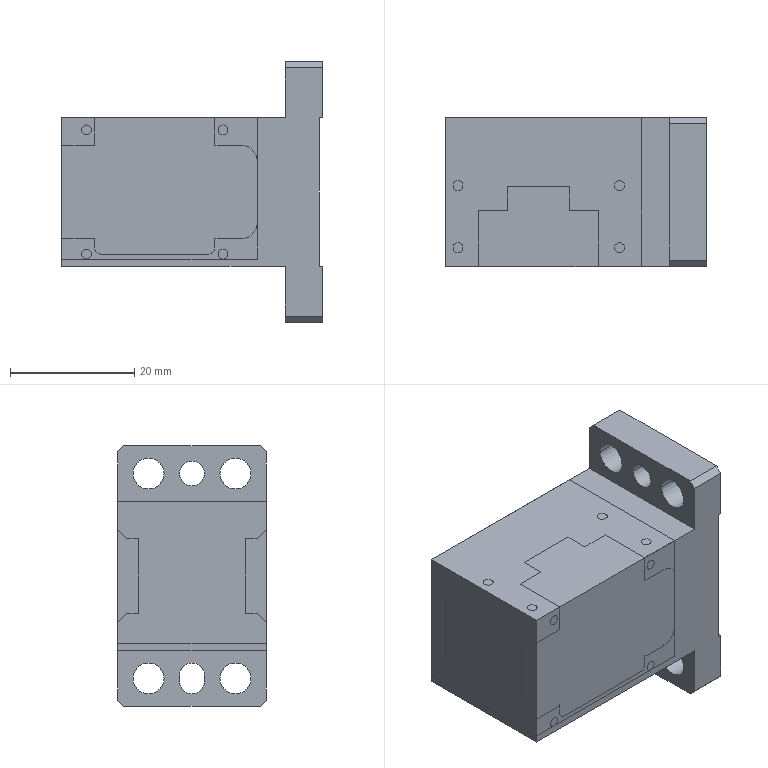NC program | NX | posted with a generic post | part box 42 x 24 x 42 mm
Lines 1 to 1189 of 31406:
N10 G17 G21 G94 G90
(CAVITY_MILL , TOOL : D6)
N12 T06 M6
N14 G54
N16 G17 G0 G90 X-16.2 Y-8.827 B0. C0. S4500 M3
N18 G43 Z30. H6
N20 Z0.902
N22 G94 G1 Z-0.098 F1000.
N24 X-12.8 Y-6.864
N26 G3 X-12.3 Y-5.998 R1.
N28 G1 X-6.3
N30 Y-6.666 F2000.
N32 G2 X0. Y-10.359 R9.165
N34 X0.9 Y-9.301 R9.109
N36 G1 Y-2.699
N38 G2 X0. Y-1.641 R9.109
N40 X-6.24 Y-5.322 R9.101
N42 G1 X-6.3 Y-5.33
N44 Y-5.998
N46 X-9.3
N48 Y-9.6
N50 X-7.403
N52 G2 X-2.372 Y-12.199 R6.165
N54 X-1.261 Y-15.7 R6.069
N56 G1 Y-18.3
N58 X1.261
N60 Y-15.693
N62 G2 X3.9 Y-10.685 R6.109
N64 G1 Y-1.315
N66 G2 X1.261 Y3.694 R6.109
N68 G1 Y4.261
N70 X-1.261
N72 Y3.695
N74 G2 X-6.625 Y-2.346 R6.101
N76 X-7.399 Y-2.4 R5.754
N78 G1 X-9.3
N80 Y-5.998
N82 X-12.3
N84 Y-12.012
N86 G3 X-15. Y-13.534 R3.7
N88 G1 Y-14.919
N90 G2 X-12. Y-12.6 R3.1
N92 G1 X-7.402
N94 G2 X-4.821 Y-13.932 R3.165
N96 X-4.261 Y-15.7 R3.069
N98 G1 Y-21.
N100 G2 X-6.597 Y-24. R3.121
N102 G1 X-5.209
N104 G3 X-3.674 Y-21.3 R3.721
N106 G1 X3.674
N108 G3 X5.209 Y-24. R3.721
N110 G1 X6.597
N112 G2 X4.261 Y-21. R3.121
N114 G1 Y-15.7
N116 G2 X6.9 Y-12.64 R3.109
N118 G1 Y0.64
N120 G2 X4.261 Y3.7 R3.109
N122 G1 Y7.261
N124 X-4.261
N126 Y3.7
N128 G2 X-7.011 Y0.629 R3.101
N130 X-7.402 Y0.6 R2.754
N132 G1 X-12.
N134 G2 X-15. Y2.919 R3.1
N136 G1 Y1.534
N138 G3 X-12.3 Y0.012 R3.7
N140 G1 Y-5.998
N142 G2 X-12.8 Y-6.864 R1.
N144 G1 X-16.2 Y-8.827
N146 Z0.902
N148 G0 Z0.804
N150 G1 Z-0.196 F1000.
N152 X-12.8 Y-6.864
N154 G3 X-12.3 Y-5.998 R1.
N156 G1 X-6.3
N158 Y-6.657 F2000.
N160 G2 X-3.357 Y-7.491 R9.284
N162 X0.001 Y-10.227 R9.096
N164 X0.9 Y-9.204 R9.111
N166 G1 Y-2.796
N168 G2 X0.001 Y-1.772 R9.112
N170 X-6.3 Y-5.34 R9.101
N172 G1 Y-5.998
N174 X-9.3
N176 Y-9.6
N178 X-7.294
N180 G2 X-4.642 Y-10.202 R6.284
N182 X-1.163 Y-15.696 R6.096
N184 G1 Y-18.3
N186 X1.163
N188 Y-15.693
N190 G2 X3.9 Y-10.619 R6.111
N192 G1 Y-1.38
N194 G2 X1.163 Y3.693 R6.112
N196 G1 Y4.163
N198 X-1.163
N200 Y3.695
N202 G2 X-6.788 Y-2.372 R6.101
N204 G1 X-7.204 Y-2.4
N206 X-9.3
N208 Y-5.998
N210 X-12.3
N212 Y-12.012
N214 G3 X-15. Y-13.534 R3.7
N216 G1 Y-14.919
N218 G2 X-12. Y-12.6 R3.1
N220 G1 X-7.304
N222 G2 X-5.926 Y-12.913 R3.284
N224 X-4.163 Y-15.7 R3.096
N226 G1 Y-21.
N228 G2 X-6.52 Y-24. R3.1
N230 G1 X-5.111
N232 G3 X-3.576 Y-21.3 R3.7
N234 G1 X3.574
N236 G3 X4.351 Y-23.274 R3.633
N238 X5.116 Y-24. R3.772
N240 G1 X6.514
N242 G2 X4.821 Y-22.901 R3.172
N244 X4.163 Y-21.014 R3.033
N246 G1 Y-15.7
N248 G2 X6.9 Y-12.626 R3.111
N250 G1 Y0.626
N252 G2 X4.163 Y3.7 R3.112
N254 G1 Y7.163
N256 X-4.163
N258 Y3.7
N260 G2 X-7.011 Y0.62 R3.101
N262 G1 X-7.304 Y0.6
N264 X-12.
N266 G2 X-15. Y2.919 R3.1
N268 G1 Y1.534
N270 G3 X-12.3 Y0.012 R3.7
N272 G1 Y-5.998
N274 G2 X-12.8 Y-6.864 R1.
N276 G1 X-16.2 Y-8.827
N278 Z0.804
N280 G0 Y-8.825 Z0.706
N282 G1 Z-0.294 F1000.
N284 X-12.8 Y-6.862
N286 G3 X-12.3 Y-5.996 R1.
N288 G1 X-6.3
N290 Y-6.645 F2000.
N292 G2 X-0.082 Y-9.996 R9.169
N294 G1 X0.001 Y-10.099
N296 G2 X0.9 Y-9.11 R9.114
N298 G1 Y-2.885
N300 G2 X0.002 Y-1.898 R9.153
N302 X-6.17 Y-5.336 R9.101
N304 G1 X-6.3 Y-5.346
N306 Y-5.996
N308 X-9.3
N310 Y-9.6
N312 X-7.207
N314 G2 X-2.412 Y-11.885 R6.169
N316 X-1.065 Y-15.687 R6.039
N318 G1 Y-18.3
N320 X1.065
N322 Y-15.692
N324 G2 X3.9 Y-10.556 R6.114
N326 G1 Y-1.439
N328 G2 X1.634 Y1.133 R6.153
N330 X1.065 Y3.679 R5.979
N332 G1 Y4.065
N334 X-1.065
N336 Y3.695
N338 G2 X-1.074 Y3.376 R6.101
N340 X-6.46 Y-2.35 R6.101
N342 G1 X-7.111 Y-2.4
N344 X-9.3
N346 Y-5.996
N348 X-12.3
N350 Y-12.012
N352 G3 X-15. Y-13.534 R3.7
N354 G1 Y-14.919
N356 G2 X-12. Y-12.6 R3.1
N358 G1 X-7.206
N360 G2 X-4.743 Y-13.774 R3.169
N362 X-4.065 Y-15.687 R3.039
N364 G1 Y-21.
N366 G2 X-6.423 Y-24. R3.099
N368 G1 X-5.013
N370 G3 X-3.478 Y-21.3 R3.699
N372 G1 X3.477
N374 G3 X5.016 Y-24. R3.682
N376 G1 X6.425
N378 G2 X5.509 Y-23.608 R3.228
N380 X4.065 Y-21. R3.082
N382 G1 Y-15.7
N384 G2 X6.9 Y-12.615 R3.114
N386 G1 Y0.615
N388 G2 X4.349 Y2.41 R3.153
N390 X4.065 Y3.679 R2.979
N392 G1 Y7.065
N394 X-4.065
N396 Y3.7
N398 G2 X-6.815 Y0.629 R3.101
N400 G1 X-6.887 Y0.62
N402 X-7.206 Y0.6
N404 X-12.
N406 G2 X-15. Y2.919 R3.1
N408 G1 Y1.534
N410 G3 X-12.3 Y0.012 R3.7
N412 G1 Y-5.996
N414 G2 X-12.8 Y-6.862 R1.
N416 G1 X-16.2 Y-8.825
N418 Z0.706
N420 G0 Y-8.828 Z0.608
N422 G1 Z-0.392 F1000.
N424 X-12.8 Y-6.865
N426 G3 X-12.3 Y-5.999 R1.
N428 G1 X-6.3
N430 Y-6.637 F2000.
N432 G2 X-1.507 Y-8.507 R9.217
N434 X0.001 Y-9.977 R9.086
N436 X0.9 Y-9.018 R9.112
N438 G1 Y-2.977
N440 G2 X0.001 Y-2.021 R9.148
N442 X-6.3 Y-5.361 R9.107
N444 G1 Y-5.999
N446 X-9.3
N448 Y-9.6
N450 X-7.102
N452 G2 X-3.336 Y-10.885 R6.217
N454 X-0.967 Y-15.698 R6.086
N456 G1 Y-18.3
N458 X0.967
N460 Y-15.693
N462 G2 X3.9 Y-10.495 R6.112
N464 G1 Y-1.5
N466 G2 X1.536 Y1.133 R6.148
N468 X0.967 Y3.68 R5.983
N470 G1 Y3.967
N472 X-0.967
N474 Y3.694
N476 G2 X-6.718 Y-2.384 R6.107
N478 G1 X-7.029 Y-2.4
N480 X-9.3
N482 Y-5.999
N484 X-12.3
N486 Y-12.012
N488 G3 X-15. Y-13.534 R3.7
N490 G1 Y-14.919
N492 G2 X-12. Y-12.6 R3.1
N494 G1 X-7.108
N496 G2 X-5.165 Y-13.262 R3.217
N498 X-3.967 Y-15.7 R3.086
N500 G1 Y-21.
N502 G2 X-6.314 Y-24. R3.132
N504 G1 X-4.923
N506 G3 X-3.381 Y-21.3 R3.732
N508 G1 X3.381
N510 G3 X4.923 Y-24. R3.732
N512 G1 X6.314
N514 G2 X3.967 Y-21. R3.132
N516 G1 Y-15.7
N518 G2 X6.9 Y-12.608 R3.112
N520 G1 Y0.608
N522 G2 X4.251 Y2.41 R3.148
N524 X3.967 Y3.68 R2.983
N526 G1 Y6.967
N528 X-3.967
N530 Y3.7
N532 G2 X-6.887 Y0.612 R3.107
N534 G1 X-7.108 Y0.6
N536 X-12.
N538 G2 X-15. Y2.919 R3.1
N540 G1 Y1.534
N542 G3 X-12.3 Y0.012 R3.7
N544 G1 Y-5.999
N546 G2 X-12.8 Y-6.865 R1.
N548 G1 X-16.2 Y-8.828
N550 Z0.608
N552 G0 Y-8.826 Z0.51
N554 G1 Z-0.49 F1000.
N556 X-12.8 Y-6.863
N558 G3 X-12.3 Y-5.997 R1.
N560 G1 X-6.3
N562 Y-6.627 F2000.
N564 G2 X-0.002 Y-9.862 R9.127
N566 X0.9 Y-8.93 R9.115
N568 G1 Y-3.071
N570 G2 X0.001 Y-2.141 R9.115
N572 X-6.3 Y-5.368 R9.105
N574 G1 Y-5.997
N576 X-9.3
N578 Y-9.6
N580 X-7.016
N582 G2 X-0.869 Y-15.687 R6.127
N584 G1 Y-18.3
N586 X0.869
N588 Y-15.692
N590 G2 X3.9 Y-10.437 R6.115
N592 G1 Y-1.563
N594 G2 X0.869 Y3.692 R6.115
N596 G1 Y3.869
N598 X-0.869
N600 Y3.694
N602 G2 X-6.653 Y-2.385 R6.105
N604 G1 X-6.927 Y-2.4
N606 X-9.3
N608 Y-5.997
N610 X-12.3
N612 Y-12.012
N614 G3 X-15. Y-13.534 R3.7
N616 G1 Y-14.919
N618 G2 X-12. Y-12.6 R3.1
N620 G1 X-7.01
N622 G2 X-3.869 Y-15.7 R3.127
N624 G1 Y-21.
N626 G2 X-6.208 Y-24. R3.124
N628 G1 X-4.819
N630 G3 X-3.283 Y-21.3 R3.724
N632 G1 X3.283
N634 G3 X4.819 Y-24. R3.724
N636 G1 X6.208
N638 G2 X3.869 Y-21. R3.124
N640 G1 Y-15.7
N642 G2 X6.9 Y-12.603 R3.115
N644 G1 Y0.603
N646 G2 X3.869 Y3.7 R3.115
N648 G1 Y6.869
N650 X-3.869
N652 Y3.7
N654 G2 X-6.814 Y0.611 R3.105
N656 G1 X-7.01 Y0.6
N658 X-12.
N660 G2 X-15. Y2.919 R3.1
N662 G1 Y1.534
N664 G3 X-12.3 Y0.012 R3.7
N666 G1 Y-5.997
N668 G2 X-12.8 Y-6.863 R1.
N670 G1 X-16.2 Y-8.826
N672 Z0.51
N674 G0 Y-8.83 Z0.412
N676 G1 Z-0.588 F1000.
N678 X-12.8 Y-6.867
N680 G3 X-12.3 Y-6.001 R1.
N682 G1 X-6.3
N684 Y-6.62 F2000.
N686 G2 X0. Y-9.743 R9.169
N688 X0.9 Y-8.842 R9.102
N690 G1 Y-3.157
N692 G2 X0. Y-2.254 R9.119
N694 X-6.3 Y-5.381 R9.121
N696 G1 Y-6.001
N698 X-9.3
N700 Y-9.6
N702 X-6.913
N704 G2 X-2.118 Y-11.885 R6.169
N706 X-0.771 Y-15.688 R6.04
N708 G1 Y-18.3
N710 X0.771
N712 Y-15.695
N714 G2 X3.9 Y-10.382 R6.102
N716 G1 Y-1.62
N718 G2 X0.771 Y3.691 R6.119
N720 G1 Y3.771
N722 X-0.771
N724 G2 X-6.921 Y-2.4 R6.121
N726 G1 X-9.3
N728 Y-6.001
N730 X-12.3
N732 Y-12.012
N734 G3 X-15. Y-13.534 R3.7
N736 G1 Y-14.919
N738 G2 X-12. Y-12.6 R3.1
N740 G1 X-6.912
N742 G2 X-4.449 Y-13.774 R3.169
N744 X-3.771 Y-15.688 R3.04
N746 G1 Y-21.
N748 G2 X-6.108 Y-24. R3.121
N750 G1 X-4.719
N752 G3 X-3.185 Y-21.3 R3.721
N754 G1 X3.185
N756 G3 X4.719 Y-24. R3.721
N758 G1 X6.108
N760 G2 X3.771 Y-21. R3.121
N762 G1 Y-15.7
N764 G2 X6.543 Y-12.626 R3.102
N766 G1 X6.9 Y-12.6
N768 Y0.6
N770 G2 X3.771 Y3.7 R3.119
N772 G1 Y6.771
N774 X-3.771
N776 Y3.7
N778 G2 X-6.912 Y0.6 R3.121
N780 G1 X-12.
N782 G2 X-15. Y2.919 R3.1
N784 G1 Y1.534
N786 G3 X-12.3 Y0.012 R3.7
N788 G1 Y-6.001
N790 G2 X-12.8 Y-6.867 R1.
N792 G1 X-16.2 Y-8.83
N794 Z0.412
N796 G0 Z0.314
N798 G1 Z-0.686 F1000.
N800 X-12.8 Y-6.867
N802 G3 X-12.3 Y-6.001 R1.
N804 G1 X-6.3
N806 Y-6.615 F2000.
N808 G2 X-0.053 Y-9.575 R9.191
N810 G1 X0.003 Y-9.637
N812 G2 X0.9 Y-8.765 R9.13
N814 G1 Y-3.238
N816 G2 X0. Y-2.363 R9.124
N818 X-6.3 Y-5.387 R9.124
N820 G1 Y-6.001
N822 X-9.3
N824 Y-9.6
N826 X-6.81
N828 G2 X-2.266 Y-11.601 R6.191
N830 X-0.673 Y-15.7 R6.071
N832 G1 Y-18.3
N834 X0.673
N836 Y-15.685
N838 G2 X3.9 Y-10.331 R6.13
N840 G1 Y-1.672
N842 G2 X0.673 Y3.673 R6.124
N844 G1 X-0.673
N846 G2 X-6.821 Y-2.4 R6.124
N848 G1 X-9.3
N850 Y-6.001
N852 X-12.3
N854 Y-12.012
N856 G3 X-15. Y-13.534 R3.7
N858 G1 Y-14.919
N860 G2 X-12. Y-12.6 R3.1
N862 G1 X-9.3
N864 X-6.809
N866 G2 X-4.476 Y-13.629 R3.191
N868 X-3.673 Y-15.7 R3.071
N870 G1 Y-21.
N872 G2 X-6.012 Y-24. R3.124
N874 G1 X-4.623
N876 G3 X-3.087 Y-21.3 R3.724
N878 G1 X3.087
N880 G3 X4.623 Y-24. R3.724
N882 G1 X6.012
N884 G2 X3.673 Y-21. R3.124
N886 G1 Y-15.7
N888 G2 X6.814 Y-12.6 R3.13
N890 G1 X6.9
N892 Y0.6
N894 X6.814
N896 G2 X3.673 Y3.7 R3.124
N898 G1 Y6.673
N900 X-3.673
N902 Y6.073
N904 Y3.677
N906 G2 X-6.814 Y0.6 R3.124
N908 G1 X-12.
N910 G2 X-15. Y2.919 R3.1
N912 G1 Y1.534
N914 G3 X-12.3 Y0.012 R3.7
N916 G1 Y-6.001
N918 G2 X-12.8 Y-6.867 R1.
N920 G1 X-16.2 Y-8.83
N922 Z0.314
N924 G0 Y-8.829 Z0.216
N926 G1 Z-0.784 F1000.
N928 X-12.8 Y-6.866
N930 G3 X-12.3 Y-6. R1.
N932 G1 X-6.3
N934 Y-6.609 F2000.
N936 G2 X0. Y-9.533 R9.13
N938 X0.9 Y-8.683 R9.13
N940 G1 Y-3.319
N942 G2 X0. Y-2.469 R9.127
N944 X-6.3 Y-5.391 R9.127
N946 G1 Y-6.
N948 X-9.3
N950 Y-9.6
N952 X-6.721
N954 G2 X-0.575 Y-15.685 R6.13
N956 G1 Y-18.3
N958 X0.575
N960 Y-15.685
N962 G2 X3.9 Y-10.28 R6.13
N964 G1 Y-1.722
N966 G2 X0.577 Y3.575 R6.127
N968 G1 X-0.577
N970 G2 X-6.722 Y-2.4 R6.127
N972 G1 X-9.3
N974 Y-6.
N976 X-12.3
N978 Y-12.012
N980 G3 X-15. Y-13.534 R3.7
N982 G1 Y-14.919
N984 G2 X-12. Y-12.6 R3.1
N986 G1 X-6.716
N988 G2 X-3.575 Y-15.7 R3.13
N990 G1 Y-21.
N992 G2 X-5.917 Y-24. R3.126
N994 G1 X-4.527
N996 G3 X-2.989 Y-21.3 R3.726
N998 G1 X2.989
N1000 G3 X4.527 Y-24. R3.726
N1002 G1 X5.917
N1004 G2 X3.575 Y-21. R3.126
N1006 G1 Y-15.7
N1008 G2 X6.716 Y-12.6 R3.13
N1010 G1 X6.9
N1012 Y0.6
N1014 X6.716
N1016 G2 X3.575 Y3.7 R3.127
N1018 G1 Y6.575
N1020 X-3.575
N1022 Y3.7
N1024 G2 X-6.716 Y0.6 R3.127
N1026 G1 X-12.
N1028 G2 X-15. Y2.919 R3.1
N1030 G1 Y1.534
N1032 G3 X-12.3 Y0.012 R3.7
N1034 G1 Y-6.
N1036 G2 X-12.8 Y-6.866 R1.
N1038 G1 X-16.2 Y-8.829
N1040 Z0.216
N1042 G0 Z0.119
N1044 G1 Z-0.881 F1000.
N1046 X-12.8 Y-6.866
N1048 G3 X-12.3 Y-6. R1.
N1050 G1 X-6.3
N1052 Y-6.605 F2000.
N1054 G2 X0. Y-9.424 R9.123
N1056 X0.9 Y-8.6 R9.123
N1058 G1 Y-3.401
N1060 G2 X0. Y-2.577 R9.121
N1062 X-6.3 Y-5.395 R9.121
N1064 G1 Y-6.
N1066 X-9.3
N1068 Y-9.6
N1070 X-6.626
N1072 G2 X-0.477 Y-15.689 R6.123
N1074 G1 Y-18.3
N1076 X0.477
N1078 Y-15.678
N1080 G2 X3.9 Y-10.227 R6.123
N1082 G1 Y-1.773
N1084 G2 X0.482 Y3.477 R6.121
N1086 G1 X-0.482
N1088 G2 X-6.627 Y-2.4 R6.121
N1090 G1 X-9.3
N1092 Y-6.
N1094 X-12.3
N1096 Y-12.012
N1098 G3 X-15. Y-13.534 R3.7
N1100 G1 Y-14.919
N1102 G2 X-12. Y-12.6 R3.1
N1104 G1 X-6.619
N1106 G2 X-3.477 Y-15.7 R3.123
N1108 G1 Y-21.
N1110 G2 X-5.815 Y-24. R3.122
N1112 G1 X-4.426
N1114 G3 X-2.891 Y-21.3 R3.722
N1116 G1 X2.891
N1118 G3 X4.425 Y-24. R3.721
N1120 G1 X5.814
N1122 G2 X3.477 Y-21. R3.121
N1124 G1 Y-18.3
N1126 Y-15.678
N1128 G2 X6.619 Y-12.6 R3.123
N1130 G1 X6.9
N1132 Y0.6
N1134 X6.619
N1136 G2 X3.477 Y3.7 R3.121
N1138 G1 Y6.477
N1140 X-3.477
N1142 Y5.877
N1144 Y3.68
N1146 G2 X-6.619 Y0.6 R3.121
N1148 G1 X-12.
N1150 G2 X-15. Y2.919 R3.1
N1152 G1 Y1.534
N1154 G3 X-12.3 Y0.012 R3.7
N1156 G1 Y-6.
N1158 G2 X-12.8 Y-6.866 R1.
N1160 G1 X-16.2 Y-8.829
N1162 Z0.119
N1164 G0 Z0.021
N1166 G1 Z-0.979 F1000.
N1168 X-12.8 Y-6.866
N1170 G3 X-12.3 Y-6. R1.
N1172 G1 X-6.3
N1174 Y-6.603 F2000.
N1176 G2 X-0.002 Y-9.322 R9.15
N1178 X0.9 Y-8.521 R9.102
N1180 G1 Y-3.479
N1182 G2 X0. Y-2.678 R9.121
N1184 X-6.3 Y-5.398 R9.121
N1186 G1 Y-6.
N1188 X-9.3
N1190 Y-9.6
N1192 X-6.523
N1194 G2 X-0.902 Y-13.236 R6.15
N1196 X-0.379 Y-15.68 R5.979
N1198 G1 Y-18.3
N1200 X0.379
N1202 Y-15.695
N1204 G2 X3.9 Y-10.181 R6.102
N1206 G1 Y-1.82
N1208 G2 X0.389 Y3.379 R6.121
N1210 G1 X-0.389
N1212 G2 X-6.529 Y-2.4 R6.121
N1214 G1 X-9.3
N1216 Y-6.
N1218 X-12.3
N1220 Y-12.012
N1222 G3 X-15. Y-13.534 R3.7
N1224 G1 Y-14.919
N1226 G2 X-12. Y-12.6 R3.1
N1228 G1 X-6.521
N1230 G2 X-3.639 Y-14.462 R3.15
N1232 X-3.379 Y-15.68 R2.979
N1234 G1 Y-21.
N1236 G2 X-5.717 Y-24. R3.122
N1238 G1 X-4.328
N1240 G3 X-2.793 Y-21.3 R3.722
N1242 G1 X2.793
N1244 G3 X4.329 Y-24. R3.723
N1246 G1 X5.718
N1248 G2 X3.379 Y-21. R3.123
N1250 G1 Y-15.7
N1252 G2 X6.145 Y-12.627 R3.102
N1254 X6.521 Y-12.6 R2.53
N1256 G1 X6.9
N1258 Y0.6
N1260 X6.521
N1262 G2 X3.379 Y3.7 R3.121
N1264 G1 Y6.379
N1266 X-3.379
N1268 Y3.7
N1270 G2 X-6.521 Y0.6 R3.121
N1272 G1 X-12.
N1274 G2 X-15. Y2.919 R3.1
N1276 G1 Y1.534
N1278 G3 X-12.3 Y0.012 R3.7
N1280 G1 Y-6.
N1282 G2 X-12.8 Y-6.866 R1.
N1284 G1 X-16.2 Y-8.829
N1286 Z0.021
N1288 G0 Z-0.077
N1290 G1 Z-1.077 F1000.
N1292 X-12.8 Y-6.866
N1294 G3 X-12.3 Y-6. R1.
N1296 G1 X-6.3
N1298 Y-6.601 F2000.
N1300 G2 X-0.81 Y-8.516 R9.207
N1302 X0. Y-9.222 R9.085
N1304 X0.9 Y-8.445 R9.101
N1306 G1 Y-3.551
N1308 G2 X0. Y-2.772 R9.127
N1310 X-6.3 Y-5.399 R9.127
N1312 G1 Y-6.
N1314 X-9.3
N1316 Y-9.6
N1318 X-6.418
N1320 G2 X-2.643 Y-10.89 R6.207
N1322 X-0.281 Y-15.698 R6.085
N1324 G1 Y-18.3
N1326 X0.281
N1328 Y-15.695
N1330 G2 X3.9 Y-10.137 R6.101
N1332 G1 Y-1.863
N1334 G2 X0.297 Y3.281 R6.127
N1336 G1 X-0.297
N1338 G2 X-6.429 Y-2.4 R6.127
N1340 G1 X-9.3
N1342 Y-6.
N1344 X-12.3
N1346 Y-12.012
N1348 G3 X-15. Y-13.534 R3.7
N1350 G1 Y-14.919
N1352 G2 X-12. Y-12.6 R3.1
N1354 G1 X-6.423
N1356 G2 X-4.476 Y-13.265 R3.207
N1358 X-3.281 Y-15.7 R3.085
N1360 G1 Y-21.
N1362 G2 X-5.638 Y-24. R3.101
N1364 G1 X-4.23
N1366 G3 X-2.694 Y-21.3 R3.701
N1368 G1 X2.692
N1370 G3 X3.317 Y-23.066 R3.625
N1372 X4.234 Y-24. R3.763
N1374 G1 X5.631
N1376 G2 X3.812 Y-22.727 R3.163
N1378 X3.281 Y-21.015 R3.025
N1380 G1 Y-15.7
N1382 G2 X6.162 Y-12.617 R3.101
N1384 G1 X6.423 Y-12.6
N1386 X6.9
N1388 Y0.6
N1390 X6.408
N1392 G2 X3.281 Y3.7 R3.127
N1394 G1 Y6.281
N1396 X-3.281
N1398 Y3.7
N1400 G2 X-6.423 Y0.6 R3.127
N1402 G1 X-12.
N1404 G2 X-15. Y2.919 R3.1
N1406 G1 Y1.534
N1408 G3 X-12.3 Y0.012 R3.7
N1410 G1 Y-6.
N1412 G2 X-12.8 Y-6.866 R1.
N1414 G1 X-16.2 Y-8.829
N1416 Z-0.077
N1418 G0 Z-0.175
N1420 G1 Z-1.175 F1000.
N1422 X-12.8 Y-6.866
N1424 G3 X-12.3 Y-6. R1.
N1426 G1 X-6.3
N1428 Y-6.6 F2000.
N1430 G2 X0. Y-9.129 R9.121
N1432 X0.9 Y-8.373 R9.121
N1434 G1 Y-3.624
N1436 G2 X0. Y-2.868 R9.126
N1438 X-6.3 Y-5.4 R9.126
N1440 G1 Y-6.
N1442 X-9.3
N1444 Y-9.6
N1446 X-6.333
N1448 G2 X-0.183 Y-15.69 R6.121
N1450 G1 Y-18.3
N1452 X0.183
N1454 Y-15.69
N1456 G2 X3.9 Y-10.092 R6.121
N1458 G1 Y-1.907
N1460 G2 X0.207 Y3.183 R6.126
N1462 G1 X-0.207
N1464 G2 X-6.331 Y-2.4 R6.126
N1466 G1 X-9.3
N1468 Y-6.
N1470 X-12.3
N1472 Y-12.012
N1474 G3 X-15. Y-13.534 R3.7
N1476 G1 Y-14.919
N1478 G2 X-12. Y-12.6 R3.1
N1480 G1 X-6.325
N1482 G2 X-3.183 Y-15.7 R3.121
N1484 G1 Y-21.
N1486 G2 X-5.523 Y-24. R3.124
N1488 G1 X-4.134
N1490 G3 X-2.597 Y-21.3 R3.724
N1492 G1 X2.597
N1494 G3 X4.134 Y-24. R3.724
N1496 G1 X5.523
N1498 G2 X3.183 Y-21. R3.124
N1500 G1 Y-15.7
N1502 G2 X6.325 Y-12.6 R3.121
N1504 G1 X6.9
N1506 Y0.6
N1508 X6.3
N1510 G2 X3.183 Y3.7 R3.126
N1512 G1 Y6.183
N1514 X-3.183
N1516 Y5.583
N1518 X-3.184 Y3.676
N1520 G2 X-6.325 Y0.6 R3.126
N1522 G1 X-12.
N1524 G2 X-15. Y2.919 R3.1
N1526 G1 Y1.534
N1528 G3 X-12.3 Y0.012 R3.7
N1530 G1 Y-6.
N1532 G2 X-12.8 Y-6.866 R1.
N1534 G1 X-16.2 Y-8.829
N1536 Z-0.175
N1538 G0 Z-0.273
N1540 G1 Z-1.273 F1000.
N1542 X-12.8 Y-6.866
N1544 G3 X-12.3 Y-6. R1.
N1546 G1 X-6.3
N1548 Y-6.6 F2000.
N1550 G2 X0. Y-9.038 R9.122
N1552 X0.9 Y-8.303 R9.122
N1554 G1 Y-3.694
N1556 G2 X0.002 Y-2.963 R9.17
N1558 X-5.314 Y-5.349 R9.101
N1560 G1 X-5.904 Y-5.394
N1562 X-6.162 Y-5.4
N1564 X-6.3
N1566 Y-6.
N1568 X-9.3
N1570 Y-9.6
N1572 X-6.234
N1574 G2 X-0.085 Y-15.689 R6.122
N1576 G1 Y-18.3
N1578 X0.085
N1580 Y-15.679
N1582 G2 X3.9 Y-10.051 R6.122
N1584 G1 Y-1.944
N1586 G2 X1.477 Y-0.168 R6.17
N1588 X0.117 Y3.085 R6.071
N1590 G1 X-0.117
N1592 G2 X-5.578 Y-2.361 R6.101
N1594 G1 X-6.051 Y-2.397
N1596 X-6.195 Y-2.4
N1598 X-9.3
N1600 Y-6.
N1602 X-12.3
N1604 Y-12.012
N1606 G3 X-15. Y-13.534 R3.7
N1608 G1 Y-14.919
N1610 G2 X-12. Y-12.6 R3.1
N1612 G1 X-6.227
N1614 G2 X-3.085 Y-15.7 R3.122
N1616 G1 Y-21.
N1618 G2 X-5.442 Y-24. R3.1
N1620 G1 X-4.033
N1622 G3 X-2.498 Y-21.3 R3.7
N1624 G1 X2.496
N1626 G3 X3.122 Y-23.067 R3.609
N1628 X4.04 Y-24. R3.773
N1630 G1 X5.439
N1632 G2 X3.616 Y-22.727 R3.173
N1634 X3.085 Y-21.02 R3.009
N1636 G1 Y-18.3
N1638 X3.086 Y-15.679
N1640 G2 X6.227 Y-12.6 R3.122
N1642 G1 X6.9
N1644 Y0.6
N1646 X6.227
N1648 G2 X3.788 Y1.745 R3.17
N1650 X3.085 Y3.7 R3.071
N1652 G1 Y6.085
N1654 X-3.085
N1656 Y3.7
N1658 G2 X-5.854 Y0.627 R3.101
N1660 G1 X-6.198 Y0.601
N1662 X-9.3 Y0.6
N1664 X-12.
N1666 G2 X-15. Y2.919 R3.1
N1668 G1 Y1.534
N1670 G3 X-12.3 Y0.012 R3.7
N1672 G1 Y-6.
N1674 G2 X-12.8 Y-6.866 R1.
N1676 G1 X-16.2 Y-8.829
N1678 Z-0.273
N1680 G0 Z-0.371
N1682 G1 Z-1.371 F1000.
N1684 X-12.8 Y-6.866
N1686 G3 X-12.3 Y-6. R1.
N1688 G1 X-6.3
N1690 Y-6.6 F2000.
N1692 X-6.165
N1694 G2 X0. Y-8.952 R9.129
N1696 X0.9 Y-8.237 R9.129
N1698 G1 Y-3.764
N1700 G2 X0. Y-3.05 R9.126
N1702 X-6.14 Y-5.4 R9.126
N1704 G1 X-6.3
N1706 Y-6.
N1708 X-9.3
N1710 Y-9.6
N1712 X-6.156
N1714 G2 X0. Y-15.334 R6.129
N1716 X3.9 Y-10.015 R6.129
N1718 G1 Y-1.986
N1720 G2 X0.032 Y2.987 R6.126
N1722 G1 X-0.032
N1724 G2 X-6.135 Y-2.4 R6.126
N1726 G1 X-9.3
N1728 Y-6.
N1730 X-12.3
N1732 Y-12.012
N1734 G3 X-15. Y-13.534 R3.7
N1736 G1 Y-14.919
N1738 G2 X-12. Y-12.6 R3.1
N1740 G1 X-6.145
N1742 G2 X-2.987 Y-15.7 R3.129
N1744 G1 Y-21.
N1746 G2 X-5.339 Y-24. R3.103
N1748 G1 X-3.934
N1750 G3 X-2.4 Y-21.3 R3.703
N1752 G1 X2.401
N1754 G3 X3.936 Y-24. R3.721
N1756 G1 X5.324
N1758 G2 X2.987 Y-21. R3.121
N1760 G1 Y-15.7
N1762 G2 X6.145 Y-12.6 R3.129
N1764 G1 X6.9
N1766 Y0.6
N1768 X6.129
N1770 G2 X2.987 Y3.7 R3.126
N1772 G1 Y5.987
N1774 X-2.987
N1776 Y3.7
N1778 G2 X-6.129 Y0.6 R3.126
N1780 G1 X-12.
N1782 G2 X-15. Y2.919 R3.1
N1784 G1 Y1.534
N1786 G3 X-12.3 Y0.012 R3.7
N1788 G1 Y-6.
N1790 G2 X-12.8 Y-6.866 R1.
N1792 G1 X-16.2 Y-8.829
N1794 Z-0.371
N1796 G0 Z-0.469
N1798 G1 Z-1.469 F1000.
N1800 X-12.8 Y-6.866
N1802 G3 X-12.3 Y-6. R1.
N1804 G1 X-6.3
N1806 Y-6.6 F2000.
N1808 X-6.04
N1810 G2 X0. Y-8.87 R9.113
N1812 X0.9 Y-8.173 R9.113
N1814 G1 Y-3.828
N1816 G2 X0.001 Y-3.132 R9.111
N1818 X-6.003 Y-5.4 R9.08
N1820 G1 X-6.3
N1822 Y-6.
N1824 X-9.3
N1826 Y-9.6
N1828 X-6.036
N1830 G2 X0. Y-14.639 R6.113
N1832 X3.9 Y-9.979 R6.113
N1834 G1 Y-2.022
N1836 G2 X-0.001 Y2.645 R6.111
N1838 X-1.31 Y-0.186 R6.158
N1840 X-6.003 Y-2.4 R6.08
N1842 G1 X-9.3
N1844 Y-6.
N1846 X-12.3
N1848 Y-12.012
N1850 G3 X-15. Y-13.534 R3.7
N1852 G1 Y-14.919
N1854 G2 X-12. Y-12.6 R3.1
N1856 G1 X-6.031
N1858 G2 X-2.905 Y-15.7 R3.113
N1860 G1 Y-20.995
N1862 G2 X-5.237 Y-24. R3.115
N1864 G1 X-3.85
N1866 G3 X-2.318 Y-21.3 R3.715
N1868 G1 X2.318
N1870 G3 X3.85 Y-24. R3.715
N1872 G1 X5.237
N1874 G2 X2.905 Y-20.995 R3.115
N1876 G1 Y-15.7
N1878 G2 X6.031 Y-12.6 R3.113
N1880 G1 X6.9
N1882 Y0.6
N1884 X6.031
N1886 G2 X2.909 Y3.561 R3.111
N1888 G1 X2.914 Y3.573
N1890 X2.908 Y3.683
N1892 X2.905 Y3.7
N1894 Y5.905
N1896 X-2.905
N1898 Y3.7
N1900 G2 X-3.625 Y1.722 R3.158
N1902 X-6.003 Y0.6 R3.08
N1904 G1 X-12.
N1906 G2 X-15. Y2.919 R3.1
N1908 G1 Y1.534
N1910 G3 X-12.3 Y0.012 R3.7
N1912 G1 Y-6.
N1914 G2 X-12.8 Y-6.866 R1.
N1916 G1 X-16.2 Y-8.829
N1918 Z-0.469
N1920 G0 Z-0.567
N1922 G1 Z-1.567 F1000.
N1924 X-12.8 Y-6.866
N1926 G3 X-12.3 Y-6. R1.
N1928 G1 X-6.3
N1930 Y-6.6 F2000.
N1932 X-6.
N1934 G2 X0. Y-8.858 R9.1
N1936 X0.9 Y-8.163 R9.1
N1938 G1 Y-3.837
N1940 G2 X0. Y-3.142 R9.1
N1942 X-6. Y-5.4 R9.1
N1944 G1 X-6.3
N1946 Y-6.
N1948 X-9.3
N1950 Y-9.6
N1952 X-6.
N1954 G2 X0. Y-14.6 R6.1
N1956 X3.9 Y-9.973 R6.1
N1958 G1 Y-2.027
N1960 G2 X0. Y2.6 R6.1
N1962 X-6. Y-2.4 R6.1
N1964 G1 X-9.3
N1966 Y-6.
N1968 X-12.3
N1970 Y-12.012
N1972 G3 X-15. Y-13.534 R3.7
N1974 G1 Y-14.919
N1976 G2 X-12. Y-12.6 R3.1
N1978 G1 X-6.
N1980 G2 X-2.9 Y-15.7 R3.1
N1982 G1 Y-21.
N1984 G2 X-5.219 Y-24. R3.1
N1986 G1 X-3.834
N1988 G3 X-2.312 Y-21.3 R3.7
N1990 G1 X2.312
N1992 G3 X3.834 Y-24. R3.7
N1994 G1 X5.219
N1996 G2 X2.9 Y-21. R3.1
N1998 G1 Y-15.7
N2000 G2 X6. Y-12.6 R3.1
N2002 G1 X6.9
N2004 Y0.6
N2006 X6.
N2008 G2 X2.9 Y3.7 R3.1
N2010 G1 Y5.9
N2012 X-2.9
N2014 Y3.7
N2016 G2 X-6. Y0.6 R3.1
N2018 G1 X-12.
N2020 G2 X-15. Y2.919 R3.1
N2022 G1 Y1.534
N2024 G3 X-12.3 Y0.012 R3.7
N2026 G1 Y-6.
N2028 G2 X-12.8 Y-6.866 R1.
N2030 G1 X-16.2 Y-8.829
N2032 Z-0.567
N2034 G0 Z-0.665
N2036 G1 Z-1.665 F1000.
N2038 X-12.8 Y-6.866
N2040 G3 X-12.3 Y-6. R1.
N2042 G1 X-6.3
N2044 Y-6.6 F2000.
N2046 X-6.
N2048 G2 X0. Y-8.858 R9.1
N2050 X0.9 Y-8.163 R9.1
N2052 G1 Y-3.837
N2054 G2 X0. Y-3.142 R9.1
N2056 X-6. Y-5.4 R9.1
N2058 G1 X-6.3
N2060 Y-6.
N2062 X-9.3
N2064 Y-9.6
N2066 X-6.
N2068 G2 X0. Y-14.6 R6.1
N2070 X3.9 Y-9.973 R6.1
N2072 G1 Y-2.027
N2074 G2 X0. Y2.6 R6.1
N2076 X-6. Y-2.4 R6.1
N2078 G1 X-9.3
N2080 Y-6.
N2082 X-12.3
N2084 Y-12.012
N2086 G3 X-15. Y-13.534 R3.7
N2088 G1 Y-14.919
N2090 G2 X-12. Y-12.6 R3.1
N2092 G1 X-6.
N2094 G2 X-2.9 Y-15.7 R3.1
N2096 G1 Y-21.
N2098 G2 X-5.219 Y-24. R3.1
N2100 G1 X-3.834
N2102 G3 X-2.312 Y-21.3 R3.7
N2104 G1 X2.312
N2106 G3 X3.834 Y-24. R3.7
N2108 G1 X5.219
N2110 G2 X2.9 Y-21. R3.1
N2112 G1 Y-15.7
N2114 G2 X6. Y-12.6 R3.1
N2116 G1 X6.9
N2118 Y0.6
N2120 X6.
N2122 G2 X2.9 Y3.7 R3.1
N2124 G1 Y5.9
N2126 X-2.9
N2128 Y3.7
N2130 G2 X-6. Y0.6 R3.1
N2132 G1 X-12.
N2134 G2 X-15. Y2.919 R3.1
N2136 G1 Y1.534
N2138 G3 X-12.3 Y0.012 R3.7
N2140 G1 Y-6.
N2142 G2 X-12.8 Y-6.866 R1.
N2144 G1 X-16.2 Y-8.829
N2146 Z-0.665
N2148 G0 Z-0.763
N2150 G1 Z-1.763 F1000.
N2152 X-12.8 Y-6.866
N2154 G3 X-12.3 Y-6. R1.
N2156 G1 X-6.3
N2158 Y-6.6 F2000.
N2160 X-6.
N2162 G2 X0. Y-8.858 R9.1
N2164 X0.9 Y-8.163 R9.1
N2166 G1 Y-3.837
N2168 G2 X0. Y-3.142 R9.1
N2170 X-6. Y-5.4 R9.1
N2172 G1 X-6.3
N2174 Y-6.
N2176 X-9.3
N2178 Y-9.6
N2180 X-6.
N2182 G2 X0. Y-14.6 R6.1
N2184 X3.9 Y-9.973 R6.1
N2186 G1 Y-2.027
N2188 G2 X0. Y2.6 R6.1
N2190 X-6. Y-2.4 R6.1
N2192 G1 X-9.3
N2194 Y-6.
N2196 X-12.3
N2198 Y-12.012
N2200 G3 X-15. Y-13.534 R3.7
N2202 G1 Y-14.919
N2204 G2 X-12. Y-12.6 R3.1
N2206 G1 X-6.
N2208 G2 X-2.9 Y-15.7 R3.1
N2210 G1 Y-21.
N2212 G2 X-5.219 Y-24. R3.1
N2214 G1 X-3.834
N2216 G3 X-2.312 Y-21.3 R3.7
N2218 G1 X2.312
N2220 G3 X3.834 Y-24. R3.7
N2222 G1 X5.219
N2224 G2 X2.9 Y-21. R3.1
N2226 G1 Y-15.7
N2228 G2 X6. Y-12.6 R3.1
N2230 G1 X6.9
N2232 Y0.6
N2234 X6.
N2236 G2 X2.9 Y3.7 R3.1
N2238 G1 Y5.9
N2240 X-2.9
N2242 Y3.7
N2244 G2 X-6. Y0.6 R3.1
N2246 G1 X-12.
N2248 G2 X-15. Y2.919 R3.1
N2250 G1 Y1.534
N2252 G3 X-12.3 Y0.012 R3.7
N2254 G1 Y-6.
N2256 G2 X-12.8 Y-6.866 R1.
N2258 G1 X-16.2 Y-8.829
N2260 Z-0.763
N2262 G0 Z-0.861
N2264 G1 Z-1.861 F1000.
N2266 X-12.8 Y-6.866
N2268 G3 X-12.3 Y-6. R1.
N2270 G1 X-6.3
N2272 Y-6.6 F2000.
N2274 X-6.
N2276 G2 X0. Y-8.858 R9.1
N2278 X0.9 Y-8.163 R9.1
N2280 G1 Y-3.837
N2282 G2 X0. Y-3.142 R9.1
N2284 X-6. Y-5.4 R9.1
N2286 G1 X-6.3
N2288 Y-6.
N2290 X-9.3
N2292 Y-9.6
N2294 X-6.
N2296 G2 X0. Y-14.6 R6.1
N2298 X3.9 Y-9.973 R6.1
N2300 G1 Y-2.027
N2302 G2 X0. Y2.6 R6.1
N2304 X-6. Y-2.4 R6.1
N2306 G1 X-9.3
N2308 Y-6.
N2310 X-12.3
N2312 Y-12.012
N2314 G3 X-15. Y-13.534 R3.7
N2316 G1 Y-14.919
N2318 G2 X-12. Y-12.6 R3.1
N2320 G1 X-6.
N2322 G2 X-2.9 Y-15.7 R3.1
N2324 G1 Y-21.
N2326 G2 X-5.219 Y-24. R3.1
N2328 G1 X-3.834
N2330 G3 X-2.312 Y-21.3 R3.7
N2332 G1 X2.312
N2334 G3 X3.834 Y-24. R3.7
N2336 G1 X5.219
N2338 G2 X2.9 Y-21. R3.1
N2340 G1 Y-15.7
N2342 G2 X6. Y-12.6 R3.1
N2344 G1 X6.9
N2346 Y0.6
N2348 X6.
N2350 G2 X2.9 Y3.7 R3.1
N2352 G1 Y5.9
N2354 X-2.9
N2356 Y3.7
N2358 G2 X-6. Y0.6 R3.1
N2360 G1 X-12.
N2362 G2 X-15. Y2.919 R3.1
N2364 G1 Y1.534
N2366 G3 X-12.3 Y0.012 R3.7
N2368 G1 Y-6.
N2370 G2 X-12.8 Y-6.866 R1.
N2372 G1 X-16.2 Y-8.829
N2374 Z-0.861
N2376 G0 Z-0.959